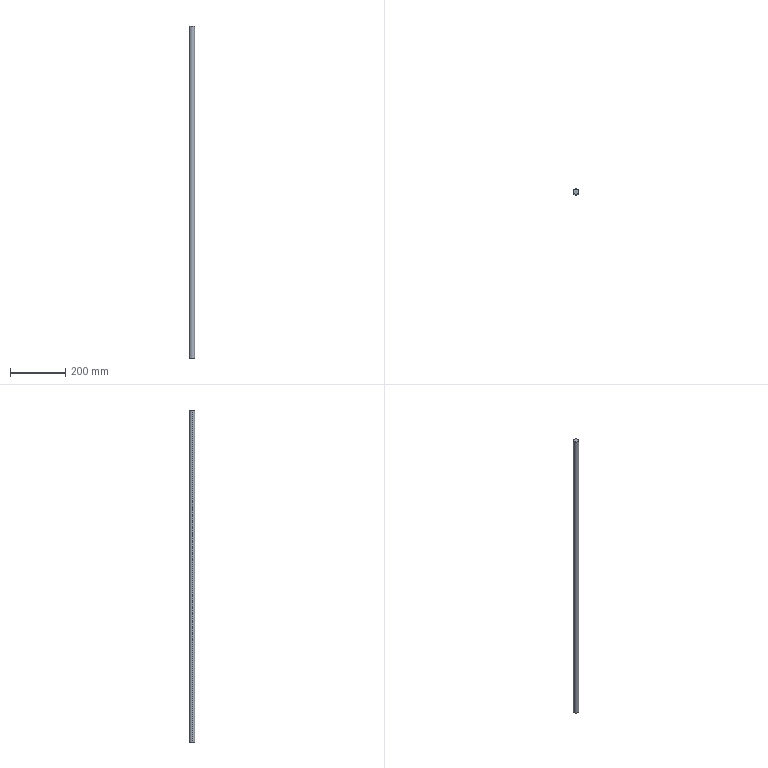Part | SolidWorks | features Extrusion 1, ICE 1 | 1 solid | 28 faces | box 20 x 20 x 1198 mm | volume 373288 mm3 | cylinder 14 | plane 14 | commonest cylinder face diameters 6 x12 20 x2
STEP:
#1=CARTESIAN_POINT('',(0.,6.5,-504.));
#2=VERTEX_POINT('',#1);
#3=CARTESIAN_POINT('',(3.,6.5,-507.));
#4=VERTEX_POINT('',#3);
#5=CARTESIAN_POINT('',(0.,6.5,-507.));
#6=DIRECTION('',(0.,1.,0.));
#7=DIRECTION('',(0.,0.,1.));
#8=AXIS2_PLACEMENT_3D('',#5,#6,#7);
#9=CIRCLE('',#8,3.);
#10=EDGE_CURVE('',#2,#4,#9,.T.);
#11=ORIENTED_EDGE('',*,*,#10,.F.);
#12=CARTESIAN_POINT('',(0.,10.,-504.));
#13=VERTEX_POINT('',#12);
#14=CARTESIAN_POINT('',(0.,6.5,-504.));
#15=DIRECTION('',(0.,1.,0.));
#16=VECTOR('',#15,1000.);
#17=LINE('',#14,#16);
#18=EDGE_CURVE('',#2,#13,#17,.T.);
#19=ORIENTED_EDGE('',*,*,#18,.T.);
#20=CARTESIAN_POINT('',(3.,9.539,-507.));
#21=VERTEX_POINT('',#20);
#22=CARTESIAN_POINT('',(3.,9.539,-507.));
#23=CARTESIAN_POINT('',(3.,9.539,-506.802));
#24=CARTESIAN_POINT('',(2.981,9.546,-506.607));
#25=CARTESIAN_POINT('',(2.904,9.569,-506.22));
#26=CARTESIAN_POINT('',(2.845,9.587,-506.029));
#27=CARTESIAN_POINT('',(2.62,9.652,-505.487));
#28=CARTESIAN_POINT('',(2.397,9.713,-505.155));
#29=CARTESIAN_POINT('',(1.985,9.802,-504.742));
#30=CARTESIAN_POINT('',(1.832,9.832,-504.616));
#31=CARTESIAN_POINT('',(1.506,9.887,-504.398));
#32=CARTESIAN_POINT('',(1.335,9.912,-504.306));
#33=CARTESIAN_POINT('',(0.973,9.954,-504.155));
#34=CARTESIAN_POINT('',(0.7814,9.971,-504.097));
#35=CARTESIAN_POINT('',(0.3955,9.994,-504.02));
#36=CARTESIAN_POINT('',(0.1994,10.,-504.));
#37=CARTESIAN_POINT('',(0.,10.,-504.));
#38=B_SPLINE_CURVE_WITH_KNOTS('',3,(#22,#23,#24,#25,#26,#27,#28,#29,#30,#31,#32,#33,#34,#35,#36,#37),.UNSPECIFIED.,.F.,.F.,(4,2,2,2,2,2,2,4),(0.01415,0.01474,0.01533,0.01651,0.0171,0.01769,0.01828,0.01887),.UNSPECIFIED.);
#39=EDGE_CURVE('',#21,#13,#38,.T.);
#40=ORIENTED_EDGE('',*,*,#39,.F.);
#41=CARTESIAN_POINT('',(3.,6.5,-507.));
#42=DIRECTION('',(0.,1.,0.));
#43=VECTOR('',#42,1000.);
#44=LINE('',#41,#43);
#45=EDGE_CURVE('',#4,#21,#44,.T.);
#46=ORIENTED_EDGE('',*,*,#45,.F.);
#47=EDGE_LOOP('',(#11,#19,#40,#46));
#48=FACE_OUTER_BOUND('',#47,.T.);
#49=CARTESIAN_POINT('',(0.,6.5,-507.));
#50=DIRECTION('',(0.,1.,0.));
#51=DIRECTION('',(0.,0.,1.));
#52=AXIS2_PLACEMENT_3D('',#49,#50,#51);
#53=CYLINDRICAL_SURFACE('',#52,3.);
#54=ADVANCED_FACE('',(#48),#53,.F.);
#55=CARTESIAN_POINT('',(0.,6.5,24.));
#56=VERTEX_POINT('',#55);
#57=CARTESIAN_POINT('',(3.,6.5,21.));
#58=VERTEX_POINT('',#57);
#59=CARTESIAN_POINT('',(0.,6.5,21.));
#60=DIRECTION('',(0.,1.,0.));
#61=DIRECTION('',(0.,0.,1.));
#62=AXIS2_PLACEMENT_3D('',#59,#60,#61);
#63=CIRCLE('',#62,3.);
#64=EDGE_CURVE('',#56,#58,#63,.T.);
#65=ORIENTED_EDGE('',*,*,#64,.F.);
#66=CARTESIAN_POINT('',(0.,10.,24.));
#67=VERTEX_POINT('',#66);
#68=CARTESIAN_POINT('',(0.,6.5,24.));
#69=DIRECTION('',(0.,1.,0.));
#70=VECTOR('',#69,1000.);
#71=LINE('',#68,#70);
#72=EDGE_CURVE('',#56,#67,#71,.T.);
#73=ORIENTED_EDGE('',*,*,#72,.T.);
#74=CARTESIAN_POINT('',(3.,9.539,21.));
#75=VERTEX_POINT('',#74);
#76=CARTESIAN_POINT('',(3.,9.539,21.));
#77=CARTESIAN_POINT('',(3.,9.539,21.198));
#78=CARTESIAN_POINT('',(2.981,9.546,21.393));
#79=CARTESIAN_POINT('',(2.904,9.569,21.78));
#80=CARTESIAN_POINT('',(2.845,9.587,21.971));
#81=CARTESIAN_POINT('',(2.62,9.652,22.513));
#82=CARTESIAN_POINT('',(2.397,9.713,22.845));
#83=CARTESIAN_POINT('',(1.985,9.802,23.258));
#84=CARTESIAN_POINT('',(1.832,9.832,23.384));
#85=CARTESIAN_POINT('',(1.506,9.887,23.602));
#86=CARTESIAN_POINT('',(1.335,9.912,23.694));
#87=CARTESIAN_POINT('',(0.973,9.954,23.845));
#88=CARTESIAN_POINT('',(0.7814,9.971,23.903));
#89=CARTESIAN_POINT('',(0.3955,9.994,23.98));
#90=CARTESIAN_POINT('',(0.1994,10.,24.));
#91=CARTESIAN_POINT('',(0.,10.,24.));
#92=B_SPLINE_CURVE_WITH_KNOTS('',3,(#76,#77,#78,#79,#80,#81,#82,#83,#84,#85,#86,#87,#88,#89,#90,#91),.UNSPECIFIED.,.F.,.F.,(4,2,2,2,2,2,2,4),(0.01415,0.01474,0.01533,0.01651,0.0171,0.01769,0.01828,0.01887),.UNSPECIFIED.);
#93=EDGE_CURVE('',#75,#67,#92,.T.);
#94=ORIENTED_EDGE('',*,*,#93,.F.);
#95=CARTESIAN_POINT('',(3.,6.5,21.));
#96=DIRECTION('',(0.,1.,0.));
#97=VECTOR('',#96,1000.);
#98=LINE('',#95,#97);
#99=EDGE_CURVE('',#58,#75,#98,.T.);
#100=ORIENTED_EDGE('',*,*,#99,.F.);
#101=EDGE_LOOP('',(#65,#73,#94,#100));
#102=FACE_OUTER_BOUND('',#101,.T.);
#103=CARTESIAN_POINT('',(0.,6.5,21.));
#104=DIRECTION('',(0.,1.,0.));
#105=DIRECTION('',(0.,0.,1.));
#106=AXIS2_PLACEMENT_3D('',#103,#104,#105);
#107=CYLINDRICAL_SURFACE('',#106,3.);
#108=ADVANCED_FACE('',(#102),#107,.F.);
#109=CARTESIAN_POINT('',(0.,6.5,-417.));
#110=VERTEX_POINT('',#109);
#111=CARTESIAN_POINT('',(3.,6.5,-420.));
#112=VERTEX_POINT('',#111);
#113=CARTESIAN_POINT('',(0.,6.5,-420.));
#114=DIRECTION('',(0.,1.,0.));
#115=DIRECTION('',(0.,0.,1.));
#116=AXIS2_PLACEMENT_3D('',#113,#114,#115);
#117=CIRCLE('',#116,3.);
#118=EDGE_CURVE('',#110,#112,#117,.T.);
#119=ORIENTED_EDGE('',*,*,#118,.F.);
#120=CARTESIAN_POINT('',(0.,10.,-417.));
#121=VERTEX_POINT('',#120);
#122=CARTESIAN_POINT('',(0.,6.5,-417.));
#123=DIRECTION('',(0.,1.,0.));
#124=VECTOR('',#123,1000.);
#125=LINE('',#122,#124);
#126=EDGE_CURVE('',#110,#121,#125,.T.);
#127=ORIENTED_EDGE('',*,*,#126,.T.);
#128=CARTESIAN_POINT('',(3.,9.539,-420.));
#129=VERTEX_POINT('',#128);
#130=CARTESIAN_POINT('',(3.,9.539,-420.));
#131=CARTESIAN_POINT('',(3.,9.539,-419.802));
#132=CARTESIAN_POINT('',(2.981,9.546,-419.607));
#133=CARTESIAN_POINT('',(2.904,9.569,-419.22));
#134=CARTESIAN_POINT('',(2.845,9.587,-419.029));
#135=CARTESIAN_POINT('',(2.62,9.652,-418.487));
#136=CARTESIAN_POINT('',(2.397,9.713,-418.155));
#137=CARTESIAN_POINT('',(1.985,9.802,-417.742));
#138=CARTESIAN_POINT('',(1.832,9.832,-417.616));
#139=CARTESIAN_POINT('',(1.506,9.887,-417.398));
#140=CARTESIAN_POINT('',(1.335,9.912,-417.306));
#141=CARTESIAN_POINT('',(0.973,9.954,-417.155));
#142=CARTESIAN_POINT('',(0.7814,9.971,-417.097));
#143=CARTESIAN_POINT('',(0.3955,9.994,-417.02));
#144=CARTESIAN_POINT('',(0.1994,10.,-417.));
#145=CARTESIAN_POINT('',(0.,10.,-417.));
#146=B_SPLINE_CURVE_WITH_KNOTS('',3,(#130,#131,#132,#133,#134,#135,#136,#137,#138,#139,#140,#141,#142,#143,#144,#145),.UNSPECIFIED.,.F.,.F.,(4,2,2,2,2,2,2,4),(0.01415,0.01474,0.01533,0.01651,0.0171,0.01769,0.01828,0.01887),.UNSPECIFIED.);
#147=EDGE_CURVE('',#129,#121,#146,.T.);
#148=ORIENTED_EDGE('',*,*,#147,.F.);
#149=CARTESIAN_POINT('',(3.,6.5,-420.));
#150=DIRECTION('',(0.,1.,0.));
#151=VECTOR('',#150,1000.);
#152=LINE('',#149,#151);
#153=EDGE_CURVE('',#112,#129,#152,.T.);
#154=ORIENTED_EDGE('',*,*,#153,.F.);
#155=EDGE_LOOP('',(#119,#127,#148,#154));
#156=FACE_OUTER_BOUND('',#155,.T.);
#157=CARTESIAN_POINT('',(0.,6.5,-420.));
#158=DIRECTION('',(0.,1.,0.));
#159=DIRECTION('',(0.,0.,1.));
#160=AXIS2_PLACEMENT_3D('',#157,#158,#159);
#161=CYLINDRICAL_SURFACE('',#160,3.);
#162=ADVANCED_FACE('',(#156),#161,.F.);
#163=CARTESIAN_POINT('',(0.,6.5,548.));
#164=VERTEX_POINT('',#163);
#165=CARTESIAN_POINT('',(3.,6.5,545.));
#166=VERTEX_POINT('',#165);
#167=CARTESIAN_POINT('',(0.,6.5,545.));
#168=DIRECTION('',(0.,1.,0.));
#169=DIRECTION('',(0.,0.,-1.));
#170=AXIS2_PLACEMENT_3D('',#167,#168,#169);
#171=CIRCLE('',#170,3.);
#172=EDGE_CURVE('',#164,#166,#171,.T.);
#173=ORIENTED_EDGE('',*,*,#172,.F.);
#174=CARTESIAN_POINT('',(0.,10.,548.));
#175=VERTEX_POINT('',#174);
#176=CARTESIAN_POINT('',(0.,6.5,548.));
#177=DIRECTION('',(0.,1.,0.));
#178=VECTOR('',#177,1000.);
#179=LINE('',#176,#178);
#180=EDGE_CURVE('',#164,#175,#179,.T.);
#181=ORIENTED_EDGE('',*,*,#180,.T.);
#182=CARTESIAN_POINT('',(3.,9.539,545.));
#183=VERTEX_POINT('',#182);
#184=CARTESIAN_POINT('',(3.,9.539,545.));
#185=CARTESIAN_POINT('',(3.,9.539,545.198));
#186=CARTESIAN_POINT('',(2.981,9.546,545.393));
#187=CARTESIAN_POINT('',(2.904,9.569,545.78));
#188=CARTESIAN_POINT('',(2.845,9.587,545.971));
#189=CARTESIAN_POINT('',(2.62,9.652,546.513));
#190=CARTESIAN_POINT('',(2.397,9.713,546.845));
#191=CARTESIAN_POINT('',(1.985,9.802,547.258));
#192=CARTESIAN_POINT('',(1.832,9.832,547.384));
#193=CARTESIAN_POINT('',(1.506,9.887,547.602));
#194=CARTESIAN_POINT('',(1.335,9.912,547.694));
#195=CARTESIAN_POINT('',(0.973,9.954,547.845));
#196=CARTESIAN_POINT('',(0.7814,9.971,547.903));
#197=CARTESIAN_POINT('',(0.3955,9.994,547.98));
#198=CARTESIAN_POINT('',(0.1994,10.,548.));
#199=CARTESIAN_POINT('',(0.,10.,548.));
#200=B_SPLINE_CURVE_WITH_KNOTS('',3,(#184,#185,#186,#187,#188,#189,#190,#191,#192,#193,#194,#195,#196,#197,#198,#199),.UNSPECIFIED.,.F.,.F.,(4,2,2,2,2,2,2,4),(0.01415,0.01474,0.01533,0.01651,0.0171,0.01769,0.01828,0.01887),.UNSPECIFIED.);
#201=EDGE_CURVE('',#183,#175,#200,.T.);
#202=ORIENTED_EDGE('',*,*,#201,.F.);
#203=CARTESIAN_POINT('',(3.,6.5,545.));
#204=DIRECTION('',(0.,1.,0.));
#205=VECTOR('',#204,1000.);
#206=LINE('',#203,#205);
#207=EDGE_CURVE('',#166,#183,#206,.T.);
#208=ORIENTED_EDGE('',*,*,#207,.F.);
#209=EDGE_LOOP('',(#173,#181,#202,#208));
#210=FACE_OUTER_BOUND('',#209,.T.);
#211=CARTESIAN_POINT('',(0.,6.5,545.));
#212=DIRECTION('',(0.,1.,0.));
#213=DIRECTION('',(0.,0.,1.));
#214=AXIS2_PLACEMENT_3D('',#211,#212,#213);
#215=CYLINDRICAL_SURFACE('',#214,3.);
#216=ADVANCED_FACE('',(#210),#215,.F.);
#217=ORIENTED_EDGE('',*,*,#39,.T.);
#218=CARTESIAN_POINT('',(-3.,9.539,-507.));
#219=VERTEX_POINT('',#218);
#220=CARTESIAN_POINT('',(0.,10.,-504.));
#221=CARTESIAN_POINT('',(-0.1995,10.,-504.));
#222=CARTESIAN_POINT('',(-0.3955,9.994,-504.02));
#223=CARTESIAN_POINT('',(-0.7806,9.971,-504.097));
#224=CARTESIAN_POINT('',(-0.9719,9.954,-504.155));
#225=CARTESIAN_POINT('',(-1.335,9.912,-504.306));
#226=CARTESIAN_POINT('',(-1.507,9.887,-504.398));
#227=CARTESIAN_POINT('',(-1.832,9.832,-504.616));
#228=CARTESIAN_POINT('',(-1.985,9.802,-504.742));
#229=CARTESIAN_POINT('',(-2.398,9.712,-505.155));
#230=CARTESIAN_POINT('',(-2.62,9.652,-505.488));
#231=CARTESIAN_POINT('',(-2.845,9.587,-506.029));
#232=CARTESIAN_POINT('',(-2.903,9.569,-506.22));
#233=CARTESIAN_POINT('',(-2.981,9.546,-506.607));
#234=CARTESIAN_POINT('',(-3.,9.539,-506.803));
#235=CARTESIAN_POINT('',(-3.,9.539,-507.));
#236=B_SPLINE_CURVE_WITH_KNOTS('',3,(#220,#221,#222,#223,#224,#225,#226,#227,#228,#229,#230,#231,#232,#233,#234,#235),.UNSPECIFIED.,.F.,.F.,(4,2,2,2,2,2,2,4),(0.,0.0005898,0.00118,0.001769,0.002359,0.003539,0.004129,0.004718),.UNSPECIFIED.);
#237=EDGE_CURVE('',#13,#219,#236,.T.);
#238=ORIENTED_EDGE('',*,*,#237,.T.);
#239=CARTESIAN_POINT('',(-3.,9.539,-545.));
#240=VERTEX_POINT('',#239);
#241=CARTESIAN_POINT('',(-3.,9.539,599.));
#242=DIRECTION('',(0.,0.,-1.));
#243=VECTOR('',#242,1000.);
#244=LINE('',#241,#243);
#245=EDGE_CURVE('',#219,#240,#244,.T.);
#246=ORIENTED_EDGE('',*,*,#245,.T.);
#247=CARTESIAN_POINT('',(3.,9.539,-545.));
#248=VERTEX_POINT('',#247);
#249=CARTESIAN_POINT('',(-3.,9.539,-545.));
#250=CARTESIAN_POINT('',(-3.,9.539,-545.197));
#251=CARTESIAN_POINT('',(-2.98,9.546,-545.397));
#252=CARTESIAN_POINT('',(-2.903,9.57,-545.783));
#253=CARTESIAN_POINT('',(-2.846,9.587,-545.97));
#254=CARTESIAN_POINT('',(-2.694,9.631,-546.335));
#255=CARTESIAN_POINT('',(-2.601,9.657,-546.508));
#256=CARTESIAN_POINT('',(-2.384,9.712,-546.832));
#257=CARTESIAN_POINT('',(-2.259,9.743,-546.984));
#258=CARTESIAN_POINT('',(-1.982,9.803,-547.261));
#259=CARTESIAN_POINT('',(-1.831,9.832,-547.384));
#260=CARTESIAN_POINT('',(-1.507,9.887,-547.601));
#261=CARTESIAN_POINT('',(-1.331,9.913,-547.695));
#262=CARTESIAN_POINT('',(-0.9699,9.955,-547.846));
#263=CARTESIAN_POINT('',(-0.7828,9.971,-547.903));
#264=CARTESIAN_POINT('',(-0.3953,9.994,-547.98));
#265=CARTESIAN_POINT('',(-0.1963,10.,-548.));
#266=CARTESIAN_POINT('',(0.1967,10.,-548.));
#267=CARTESIAN_POINT('',(0.3937,9.994,-547.981));
#268=CARTESIAN_POINT('',(0.7832,9.971,-547.903));
#269=CARTESIAN_POINT('',(0.9708,9.954,-547.845));
#270=CARTESIAN_POINT('',(1.332,9.913,-547.695));
#271=CARTESIAN_POINT('',(1.508,9.887,-547.601));
#272=CARTESIAN_POINT('',(1.833,9.832,-547.383));
#273=CARTESIAN_POINT('',(1.983,9.802,-547.26));
#274=CARTESIAN_POINT('',(2.26,9.742,-546.983));
#275=CARTESIAN_POINT('',(2.385,9.712,-546.83));
#276=CARTESIAN_POINT('',(2.601,9.656,-546.507));
#277=CARTESIAN_POINT('',(2.694,9.631,-546.335));
#278=CARTESIAN_POINT('',(2.846,9.587,-545.969));
#279=CARTESIAN_POINT('',(2.903,9.569,-545.782));
#280=CARTESIAN_POINT('',(2.98,9.546,-545.397));
#281=CARTESIAN_POINT('',(3.,9.539,-545.198));
#282=CARTESIAN_POINT('',(3.,9.539,-545.));
#283=B_SPLINE_CURVE_WITH_KNOTS('',3,(#249,#250,#251,#252,#253,#254,#255,#256,#257,#258,#259,#260,#261,#262,#263,#264,#265,#266,#267,#268,#269,#270,#271,#272,#273,#274,#275,#276,#277,#278,#279,#280,#281,#282),.UNSPECIFIED.,.F.,.F.,(4,2,2,2,2,2,2,2,2,2,2,2,2,2,2,2,4),(0.004718,0.005308,0.005897,0.006487,0.007076,0.007666,0.008255,0.008845,0.009434,0.01002,0.01061,0.0112,0.01179,0.01238,0.01297,0.01356,0.01415),.UNSPECIFIED.);
#284=EDGE_CURVE('',#240,#248,#283,.T.);
#285=ORIENTED_EDGE('',*,*,#284,.T.);
#286=CARTESIAN_POINT('',(3.,9.539,599.));
#287=DIRECTION('',(0.,0.,1.));
#288=VECTOR('',#287,1000.);
#289=LINE('',#286,#288);
#290=EDGE_CURVE('',#248,#21,#289,.T.);
#291=ORIENTED_EDGE('',*,*,#290,.T.);
#292=EDGE_LOOP('',(#217,#238,#246,#285,#291));
#293=FACE_BOUND('',#292,.T.);
#294=ORIENTED_EDGE('',*,*,#93,.T.);
#295=CARTESIAN_POINT('',(-3.,9.539,21.));
#296=VERTEX_POINT('',#295);
#297=CARTESIAN_POINT('',(0.,10.,24.));
#298=CARTESIAN_POINT('',(-0.1995,10.,24.));
#299=CARTESIAN_POINT('',(-0.3955,9.994,23.98));
#300=CARTESIAN_POINT('',(-0.7806,9.971,23.903));
#301=CARTESIAN_POINT('',(-0.9719,9.954,23.845));
#302=CARTESIAN_POINT('',(-1.335,9.912,23.694));
#303=CARTESIAN_POINT('',(-1.507,9.887,23.602));
#304=CARTESIAN_POINT('',(-1.832,9.832,23.384));
#305=CARTESIAN_POINT('',(-1.985,9.802,23.258));
#306=CARTESIAN_POINT('',(-2.398,9.712,22.845));
#307=CARTESIAN_POINT('',(-2.62,9.652,22.512));
#308=CARTESIAN_POINT('',(-2.845,9.587,21.971));
#309=CARTESIAN_POINT('',(-2.903,9.569,21.78));
#310=CARTESIAN_POINT('',(-2.981,9.546,21.393));
#311=CARTESIAN_POINT('',(-3.,9.539,21.197));
#312=CARTESIAN_POINT('',(-3.,9.539,21.));
#313=B_SPLINE_CURVE_WITH_KNOTS('',3,(#297,#298,#299,#300,#301,#302,#303,#304,#305,#306,#307,#308,#309,#310,#311,#312),.UNSPECIFIED.,.F.,.F.,(4,2,2,2,2,2,2,4),(0.,0.0005898,0.00118,0.001769,0.002359,0.003539,0.004129,0.004718),.UNSPECIFIED.);
#314=EDGE_CURVE('',#67,#296,#313,.T.);
#315=ORIENTED_EDGE('',*,*,#314,.T.);
#316=CARTESIAN_POINT('',(-3.,9.539,-17.));
#317=VERTEX_POINT('',#316);
#318=CARTESIAN_POINT('',(-3.,9.539,599.));
#319=DIRECTION('',(0.,0.,-1.));
#320=VECTOR('',#319,1000.);
#321=LINE('',#318,#320);
#322=EDGE_CURVE('',#296,#317,#321,.T.);
#323=ORIENTED_EDGE('',*,*,#322,.T.);
#324=CARTESIAN_POINT('',(3.,9.539,-17.));
#325=VERTEX_POINT('',#324);
#326=CARTESIAN_POINT('',(-3.,9.539,-17.));
#327=CARTESIAN_POINT('',(-3.,9.539,-17.197));
#328=CARTESIAN_POINT('',(-2.98,9.546,-17.397));
#329=CARTESIAN_POINT('',(-2.903,9.57,-17.783));
#330=CARTESIAN_POINT('',(-2.846,9.587,-17.97));
#331=CARTESIAN_POINT('',(-2.694,9.631,-18.335));
#332=CARTESIAN_POINT('',(-2.601,9.657,-18.508));
#333=CARTESIAN_POINT('',(-2.384,9.712,-18.832));
#334=CARTESIAN_POINT('',(-2.259,9.743,-18.984));
#335=CARTESIAN_POINT('',(-1.982,9.803,-19.261));
#336=CARTESIAN_POINT('',(-1.831,9.832,-19.384));
#337=CARTESIAN_POINT('',(-1.507,9.887,-19.601));
#338=CARTESIAN_POINT('',(-1.331,9.913,-19.695));
#339=CARTESIAN_POINT('',(-0.9699,9.955,-19.846));
#340=CARTESIAN_POINT('',(-0.7828,9.971,-19.903));
#341=CARTESIAN_POINT('',(-0.3953,9.994,-19.98));
#342=CARTESIAN_POINT('',(-0.1963,10.,-20.));
#343=CARTESIAN_POINT('',(0.1967,10.,-20.));
#344=CARTESIAN_POINT('',(0.3937,9.994,-19.981));
#345=CARTESIAN_POINT('',(0.7832,9.971,-19.903));
#346=CARTESIAN_POINT('',(0.9708,9.954,-19.845));
#347=CARTESIAN_POINT('',(1.332,9.913,-19.695));
#348=CARTESIAN_POINT('',(1.508,9.887,-19.601));
#349=CARTESIAN_POINT('',(1.833,9.832,-19.383));
#350=CARTESIAN_POINT('',(1.983,9.802,-19.26));
#351=CARTESIAN_POINT('',(2.26,9.742,-18.983));
#352=CARTESIAN_POINT('',(2.385,9.712,-18.83));
#353=CARTESIAN_POINT('',(2.601,9.656,-18.507));
#354=CARTESIAN_POINT('',(2.694,9.631,-18.335));
#355=CARTESIAN_POINT('',(2.846,9.587,-17.969));
#356=CARTESIAN_POINT('',(2.903,9.569,-17.782));
#357=CARTESIAN_POINT('',(2.98,9.546,-17.397));
#358=CARTESIAN_POINT('',(3.,9.539,-17.198));
#359=CARTESIAN_POINT('',(3.,9.539,-17.));
#360=B_SPLINE_CURVE_WITH_KNOTS('',3,(#326,#327,#328,#329,#330,#331,#332,#333,#334,#335,#336,#337,#338,#339,#340,#341,#342,#343,#344,#345,#346,#347,#348,#349,#350,#351,#352,#353,#354,#355,#356,#357,#358,#359),.UNSPECIFIED.,.F.,.F.,(4,2,2,2,2,2,2,2,2,2,2,2,2,2,2,2,4),(0.004718,0.005308,0.005897,0.006487,0.007076,0.007666,0.008255,0.008845,0.009434,0.01002,0.01061,0.0112,0.01179,0.01238,0.01297,0.01356,0.01415),.UNSPECIFIED.);
#361=EDGE_CURVE('',#317,#325,#360,.T.);
#362=ORIENTED_EDGE('',*,*,#361,.T.);
#363=CARTESIAN_POINT('',(3.,9.539,599.));
#364=DIRECTION('',(0.,0.,1.));
#365=VECTOR('',#364,1000.);
#366=LINE('',#363,#365);
#367=EDGE_CURVE('',#325,#75,#366,.T.);
#368=ORIENTED_EDGE('',*,*,#367,.T.);
#369=EDGE_LOOP('',(#294,#315,#323,#362,#368));
#370=FACE_BOUND('',#369,.T.);
#371=ORIENTED_EDGE('',*,*,#147,.T.);
#372=CARTESIAN_POINT('',(-3.,9.539,-420.));
#373=VERTEX_POINT('',#372);
#374=CARTESIAN_POINT('',(0.,10.,-417.));
#375=CARTESIAN_POINT('',(-0.1995,10.,-417.));
#376=CARTESIAN_POINT('',(-0.3955,9.994,-417.02));
#377=CARTESIAN_POINT('',(-0.7806,9.971,-417.097));
#378=CARTESIAN_POINT('',(-0.9719,9.954,-417.155));
#379=CARTESIAN_POINT('',(-1.335,9.912,-417.306));
#380=CARTESIAN_POINT('',(-1.507,9.887,-417.398));
#381=CARTESIAN_POINT('',(-1.832,9.832,-417.616));
#382=CARTESIAN_POINT('',(-1.985,9.802,-417.742));
#383=CARTESIAN_POINT('',(-2.398,9.712,-418.155));
#384=CARTESIAN_POINT('',(-2.62,9.652,-418.488));
#385=CARTESIAN_POINT('',(-2.845,9.587,-419.029));
#386=CARTESIAN_POINT('',(-2.903,9.569,-419.22));
#387=CARTESIAN_POINT('',(-2.981,9.546,-419.607));
#388=CARTESIAN_POINT('',(-3.,9.539,-419.803));
#389=CARTESIAN_POINT('',(-3.,9.539,-420.));
#390=B_SPLINE_CURVE_WITH_KNOTS('',3,(#374,#375,#376,#377,#378,#379,#380,#381,#382,#383,#384,#385,#386,#387,#388,#389),.UNSPECIFIED.,.F.,.F.,(4,2,2,2,2,2,2,4),(0.,0.0005898,0.00118,0.001769,0.002359,0.003539,0.004129,0.004718),.UNSPECIFIED.);
#391=EDGE_CURVE('',#121,#373,#390,.T.);
#392=ORIENTED_EDGE('',*,*,#391,.T.);
#393=CARTESIAN_POINT('',(-3.,9.539,-440.));
#394=VERTEX_POINT('',#393);
#395=CARTESIAN_POINT('',(-3.,9.539,599.));
#396=DIRECTION('',(0.,0.,-1.));
#397=VECTOR('',#396,1000.);
#398=LINE('',#395,#397);
#399=EDGE_CURVE('',#373,#394,#398,.T.);
#400=ORIENTED_EDGE('',*,*,#399,.T.);
#401=CARTESIAN_POINT('',(3.,9.539,-440.));
#402=VERTEX_POINT('',#401);
#403=CARTESIAN_POINT('',(-3.,9.539,-440.));
#404=CARTESIAN_POINT('',(-3.,9.539,-440.199));
#405=CARTESIAN_POINT('',(-2.98,9.546,-440.395));
#406=CARTESIAN_POINT('',(-2.903,9.569,-440.78));
#407=CARTESIAN_POINT('',(-2.845,9.587,-440.971));
#408=CARTESIAN_POINT('',(-2.694,9.631,-441.334));
#409=CARTESIAN_POINT('',(-2.602,9.656,-441.506));
#410=CARTESIAN_POINT('',(-2.385,9.712,-441.831));
#411=CARTESIAN_POINT('',(-2.259,9.743,-441.984));
#412=CARTESIAN_POINT('',(-1.847,9.832,-442.396));
#413=CARTESIAN_POINT('',(-1.514,9.891,-442.619));
#414=CARTESIAN_POINT('',(-0.9732,9.954,-442.844));
#415=CARTESIAN_POINT('',(-0.783,9.971,-442.903));
#416=CARTESIAN_POINT('',(-0.3953,9.994,-442.98));
#417=CARTESIAN_POINT('',(-0.1999,10.,-443.));
#418=CARTESIAN_POINT('',(0.194,10.,-443.));
#419=CARTESIAN_POINT('',(0.394,9.994,-442.981));
#420=CARTESIAN_POINT('',(0.7797,9.971,-442.904));
#421=CARTESIAN_POINT('',(0.9673,9.955,-442.847));
#422=CARTESIAN_POINT('',(1.332,9.913,-442.695));
#423=CARTESIAN_POINT('',(1.506,9.887,-442.602));
#424=CARTESIAN_POINT('',(1.83,9.833,-442.386));
#425=CARTESIAN_POINT('',(1.982,9.803,-442.26));
#426=CARTESIAN_POINT('',(2.259,9.743,-441.984));
#427=CARTESIAN_POINT('',(2.383,9.713,-441.833));
#428=CARTESIAN_POINT('',(2.6,9.657,-441.51));
#429=CARTESIAN_POINT('',(2.694,9.631,-441.334));
#430=CARTESIAN_POINT('',(2.845,9.587,-440.973));
#431=CARTESIAN_POINT('',(2.902,9.57,-440.786));
#432=CARTESIAN_POINT('',(2.98,9.546,-440.399));
#433=CARTESIAN_POINT('',(3.,9.539,-440.199));
#434=CARTESIAN_POINT('',(3.,9.539,-440.));
#435=B_SPLINE_CURVE_WITH_KNOTS('',3,(#403,#404,#405,#406,#407,#408,#409,#410,#411,#412,#413,#414,#415,#416,#417,#418,#419,#420,#421,#422,#423,#424,#425,#426,#427,#428,#429,#430,#431,#432,#433,#434),.UNSPECIFIED.,.F.,.F.,(4,2,2,2,2,2,2,2,2,2,2,2,2,2,2,4),(0.,0.0005894,0.001179,0.001768,0.002358,0.003536,0.004126,0.004715,0.005305,0.005894,0.006484,0.007073,0.007662,0.008252,0.008841,0.009431),.UNSPECIFIED.);
#436=EDGE_CURVE('',#394,#402,#435,.T.);
#437=ORIENTED_EDGE('',*,*,#436,.T.);
#438=CARTESIAN_POINT('',(3.,9.539,599.));
#439=DIRECTION('',(0.,0.,1.));
#440=VECTOR('',#439,1000.);
#441=LINE('',#438,#440);
#442=EDGE_CURVE('',#402,#129,#441,.T.);
#443=ORIENTED_EDGE('',*,*,#442,.T.);
#444=EDGE_LOOP('',(#371,#392,#400,#437,#443));
#445=FACE_BOUND('',#444,.T.);
#446=ORIENTED_EDGE('',*,*,#201,.T.);
#447=CARTESIAN_POINT('',(-3.,9.539,545.));
#448=VERTEX_POINT('',#447);
#449=CARTESIAN_POINT('',(0.,10.,548.));
#450=CARTESIAN_POINT('',(-0.1995,10.,548.));
#451=CARTESIAN_POINT('',(-0.3955,9.994,547.98));
#452=CARTESIAN_POINT('',(-0.7806,9.971,547.903));
#453=CARTESIAN_POINT('',(-0.9719,9.954,547.845));
#454=CARTESIAN_POINT('',(-1.335,9.912,547.694));
#455=CARTESIAN_POINT('',(-1.507,9.887,547.602));
#456=CARTESIAN_POINT('',(-1.832,9.832,547.384));
#457=CARTESIAN_POINT('',(-1.985,9.802,547.258));
#458=CARTESIAN_POINT('',(-2.398,9.712,546.845));
#459=CARTESIAN_POINT('',(-2.62,9.652,546.512));
#460=CARTESIAN_POINT('',(-2.845,9.587,545.971));
#461=CARTESIAN_POINT('',(-2.903,9.569,545.78));
#462=CARTESIAN_POINT('',(-2.981,9.546,545.393));
#463=CARTESIAN_POINT('',(-3.,9.539,545.197));
#464=CARTESIAN_POINT('',(-3.,9.539,545.));
#465=B_SPLINE_CURVE_WITH_KNOTS('',3,(#449,#450,#451,#452,#453,#454,#455,#456,#457,#458,#459,#460,#461,#462,#463,#464),.UNSPECIFIED.,.F.,.F.,(4,2,2,2,2,2,2,4),(0.,0.0005898,0.00118,0.001769,0.002359,0.003539,0.004129,0.004718),.UNSPECIFIED.);
#466=EDGE_CURVE('',#175,#448,#465,.T.);
#467=ORIENTED_EDGE('',*,*,#466,.T.);
#468=CARTESIAN_POINT('',(-3.,9.539,507.));
#469=VERTEX_POINT('',#468);
#470=CARTESIAN_POINT('',(-3.,9.539,599.));
#471=DIRECTION('',(0.,0.,-1.));
#472=VECTOR('',#471,1000.);
#473=LINE('',#470,#472);
#474=EDGE_CURVE('',#448,#469,#473,.T.);
#475=ORIENTED_EDGE('',*,*,#474,.T.);
#476=CARTESIAN_POINT('',(3.,9.539,507.));
#477=VERTEX_POINT('',#476);
#478=CARTESIAN_POINT('',(-3.,9.539,507.));
#479=CARTESIAN_POINT('',(-3.,9.539,506.801));
#480=CARTESIAN_POINT('',(-2.98,9.546,506.605));
#481=CARTESIAN_POINT('',(-2.903,9.569,506.22));
#482=CARTESIAN_POINT('',(-2.845,9.587,506.029));
#483=CARTESIAN_POINT('',(-2.694,9.631,505.666));
#484=CARTESIAN_POINT('',(-2.602,9.656,505.494));
#485=CARTESIAN_POINT('',(-2.385,9.712,505.169));
#486=CARTESIAN_POINT('',(-2.259,9.743,505.016));
#487=CARTESIAN_POINT('',(-1.847,9.832,504.604));
#488=CARTESIAN_POINT('',(-1.514,9.891,504.381));
#489=CARTESIAN_POINT('',(-0.9732,9.954,504.156));
#490=CARTESIAN_POINT('',(-0.783,9.971,504.097));
#491=CARTESIAN_POINT('',(-0.3953,9.994,504.02));
#492=CARTESIAN_POINT('',(-0.1999,10.,504.));
#493=CARTESIAN_POINT('',(0.194,10.,504.));
#494=CARTESIAN_POINT('',(0.394,9.994,504.019));
#495=CARTESIAN_POINT('',(0.7797,9.971,504.096));
#496=CARTESIAN_POINT('',(0.9673,9.955,504.153));
#497=CARTESIAN_POINT('',(1.332,9.913,504.305));
#498=CARTESIAN_POINT('',(1.506,9.887,504.398));
#499=CARTESIAN_POINT('',(1.83,9.833,504.614));
#500=CARTESIAN_POINT('',(1.982,9.803,504.74));
#501=CARTESIAN_POINT('',(2.259,9.743,505.016));
#502=CARTESIAN_POINT('',(2.383,9.713,505.167));
#503=CARTESIAN_POINT('',(2.6,9.657,505.49));
#504=CARTESIAN_POINT('',(2.694,9.631,505.666));
#505=CARTESIAN_POINT('',(2.845,9.587,506.027));
#506=CARTESIAN_POINT('',(2.902,9.57,506.214));
#507=CARTESIAN_POINT('',(2.98,9.546,506.601));
#508=CARTESIAN_POINT('',(3.,9.539,506.801));
#509=CARTESIAN_POINT('',(3.,9.539,507.));
#510=B_SPLINE_CURVE_WITH_KNOTS('',3,(#478,#479,#480,#481,#482,#483,#484,#485,#486,#487,#488,#489,#490,#491,#492,#493,#494,#495,#496,#497,#498,#499,#500,#501,#502,#503,#504,#505,#506,#507,#508,#509),.UNSPECIFIED.,.F.,.F.,(4,2,2,2,2,2,2,2,2,2,2,2,2,2,2,4),(0.,0.0005894,0.001179,0.001768,0.002358,0.003536,0.004126,0.004715,0.005305,0.005894,0.006484,0.007073,0.007662,0.008252,0.008841,0.009431),.UNSPECIFIED.);
#511=EDGE_CURVE('',#469,#477,#510,.T.);
#512=ORIENTED_EDGE('',*,*,#511,.T.);
#513=CARTESIAN_POINT('',(3.,9.539,599.));
#514=DIRECTION('',(0.,0.,1.));
#515=VECTOR('',#514,1000.);
#516=LINE('',#513,#515);
#517=EDGE_CURVE('',#477,#183,#516,.T.);
#518=ORIENTED_EDGE('',*,*,#517,.T.);
#519=EDGE_LOOP('',(#446,#467,#475,#512,#518));
#520=FACE_BOUND('',#519,.T.);
#521=CARTESIAN_POINT('',(10.,0.,599.));
#522=VERTEX_POINT('',#521);
#523=CARTESIAN_POINT('',(-10.,0.,599.));
#524=VERTEX_POINT('',#523);
#525=CARTESIAN_POINT('',(0.,0.,599.));
#526=DIRECTION('',(0.,0.,1.));
#527=DIRECTION('',(1.,0.,0.));
#528=AXIS2_PLACEMENT_3D('',#525,#526,#527);
#529=CIRCLE('',#528,10.);
#530=EDGE_CURVE('',#522,#524,#529,.T.);
#531=ORIENTED_EDGE('',*,*,#530,.F.);
#532=CARTESIAN_POINT('',(10.,0.,-599.));
#533=VERTEX_POINT('',#532);
#534=CARTESIAN_POINT('',(10.,0.,599.));
#535=DIRECTION('',(0.,0.,-1.));
#536=VECTOR('',#535,1000.);
#537=LINE('',#534,#536);
#538=EDGE_CURVE('',#522,#533,#537,.T.);
#539=ORIENTED_EDGE('',*,*,#538,.T.);
#540=CARTESIAN_POINT('',(-10.,0.,-599.));
#541=VERTEX_POINT('',#540);
#542=CARTESIAN_POINT('',(0.,0.,-599.));
#543=DIRECTION('',(0.,0.,1.));
#544=DIRECTION('',(1.,0.,0.));
#545=AXIS2_PLACEMENT_3D('',#542,#543,#544);
#546=CIRCLE('',#545,10.);
#547=EDGE_CURVE('',#533,#541,#546,.T.);
#548=ORIENTED_EDGE('',*,*,#547,.T.);
#549=CARTESIAN_POINT('',(-10.,0.,599.));
#550=DIRECTION('',(0.,0.,-1.));
#551=VECTOR('',#550,1000.);
#552=LINE('',#549,#551);
#553=EDGE_CURVE('',#524,#541,#552,.T.);
#554=ORIENTED_EDGE('',*,*,#553,.F.);
#555=EDGE_LOOP('',(#531,#539,#548,#554));
#556=FACE_OUTER_BOUND('',#555,.T.);
#557=CARTESIAN_POINT('',(0.,0.,599.));
#558=DIRECTION('',(0.,0.,-1.));
#559=DIRECTION('',(-1.,0.,0.));
#560=AXIS2_PLACEMENT_3D('',#557,#558,#559);
#561=CYLINDRICAL_SURFACE('',#560,10.);
#562=ADVANCED_FACE('',(#293,#370,#445,#520,#556),#561,.T.);
#563=ORIENTED_EDGE('',*,*,#538,.F.);
#564=CARTESIAN_POINT('',(0.,0.,599.));
#565=DIRECTION('',(0.,0.,1.));
#566=DIRECTION('',(1.,0.,0.));
#567=AXIS2_PLACEMENT_3D('',#564,#565,#566);
#568=CIRCLE('',#567,10.);
#569=EDGE_CURVE('',#524,#522,#568,.T.);
#570=ORIENTED_EDGE('',*,*,#569,.F.);
#571=ORIENTED_EDGE('',*,*,#553,.T.);
#572=CARTESIAN_POINT('',(0.,0.,-599.));
#573=DIRECTION('',(0.,0.,1.));
#574=DIRECTION('',(1.,0.,0.));
#575=AXIS2_PLACEMENT_3D('',#572,#573,#574);
#576=CIRCLE('',#575,10.);
#577=EDGE_CURVE('',#541,#533,#576,.T.);
#578=ORIENTED_EDGE('',*,*,#577,.T.);
#579=EDGE_LOOP('',(#563,#570,#571,#578));
#580=FACE_OUTER_BOUND('',#579,.T.);
#581=CARTESIAN_POINT('',(0.,0.,599.));
#582=DIRECTION('',(0.,0.,-1.));
#583=DIRECTION('',(-1.,0.,0.));
#584=AXIS2_PLACEMENT_3D('',#581,#582,#583);
#585=CYLINDRICAL_SURFACE('',#584,10.);
#586=ADVANCED_FACE('',(#580),#585,.T.);
#587=ORIENTED_EDGE('',*,*,#569,.T.);
#588=ORIENTED_EDGE('',*,*,#530,.T.);
#589=EDGE_LOOP('',(#587,#588));
#590=FACE_OUTER_BOUND('',#589,.T.);
#591=CARTESIAN_POINT('',(0.,0.,599.));
#592=DIRECTION('',(0.,0.,1.));
#593=DIRECTION('',(1.,0.,0.));
#594=AXIS2_PLACEMENT_3D('',#591,#592,#593);
#595=PLANE('',#594);
#596=ADVANCED_FACE('',(#590),#595,.T.);
#597=ORIENTED_EDGE('',*,*,#577,.F.);
#598=ORIENTED_EDGE('',*,*,#547,.F.);
#599=EDGE_LOOP('',(#597,#598));
#600=FACE_OUTER_BOUND('',#599,.T.);
#601=CARTESIAN_POINT('',(0.,0.,-599.));
#602=DIRECTION('',(0.,0.,1.));
#603=DIRECTION('',(1.,0.,0.));
#604=AXIS2_PLACEMENT_3D('',#601,#602,#603);
#605=PLANE('',#604);
#606=ADVANCED_FACE('',(#600),#605,.F.);
#607=CARTESIAN_POINT('',(-3.,6.5,507.));
#608=VERTEX_POINT('',#607);
#609=CARTESIAN_POINT('',(-3.,6.5,507.));
#610=DIRECTION('',(0.,1.,0.));
#611=VECTOR('',#610,1000.);
#612=LINE('',#609,#611);
#613=EDGE_CURVE('',#608,#469,#612,.T.);
#614=ORIENTED_EDGE('',*,*,#613,.F.);
#615=CARTESIAN_POINT('',(3.,6.5,507.));
#616=VERTEX_POINT('',#615);
#617=CARTESIAN_POINT('',(0.,6.5,507.));
#618=DIRECTION('',(0.,1.,0.));
#619=DIRECTION('',(0.,0.,-1.));
#620=AXIS2_PLACEMENT_3D('',#617,#618,#619);
#621=CIRCLE('',#620,3.);
#622=EDGE_CURVE('',#616,#608,#621,.T.);
#623=ORIENTED_EDGE('',*,*,#622,.F.);
#624=CARTESIAN_POINT('',(3.,6.5,507.));
#625=DIRECTION('',(0.,1.,0.));
#626=VECTOR('',#625,1000.);
#627=LINE('',#624,#626);
#628=EDGE_CURVE('',#616,#477,#627,.T.);
#629=ORIENTED_EDGE('',*,*,#628,.T.);
#630=ORIENTED_EDGE('',*,*,#511,.F.);
#631=EDGE_LOOP('',(#614,#623,#629,#630));
#632=FACE_OUTER_BOUND('',#631,.T.);
#633=CARTESIAN_POINT('',(0.,6.5,507.));
#634=DIRECTION('',(0.,1.,0.));
#635=DIRECTION('',(0.,0.,1.));
#636=AXIS2_PLACEMENT_3D('',#633,#634,#635);
#637=CYLINDRICAL_SURFACE('',#636,3.);
#638=ADVANCED_FACE('',(#632),#637,.F.);
#639=ORIENTED_EDGE('',*,*,#628,.F.);
#640=CARTESIAN_POINT('',(3.,6.5,507.));
#641=DIRECTION('',(0.,0.,-1.));
#642=VECTOR('',#641,1000.);
#643=LINE('',#640,#642);
#644=EDGE_CURVE('',#166,#616,#643,.T.);
#645=ORIENTED_EDGE('',*,*,#644,.F.);
#646=ORIENTED_EDGE('',*,*,#207,.T.);
#647=ORIENTED_EDGE('',*,*,#517,.F.);
#648=EDGE_LOOP('',(#639,#645,#646,#647));
#649=FACE_OUTER_BOUND('',#648,.T.);
#650=CARTESIAN_POINT('',(3.,6.5,507.));
#651=DIRECTION('',(1.,0.,0.));
#652=DIRECTION('',(0.,0.,-1.));
#653=AXIS2_PLACEMENT_3D('',#650,#651,#652);
#654=PLANE('',#653);
#655=ADVANCED_FACE('',(#649),#654,.F.);
#656=ORIENTED_EDGE('',*,*,#180,.F.);
#657=CARTESIAN_POINT('',(-3.,6.5,545.));
#658=VERTEX_POINT('',#657);
#659=CARTESIAN_POINT('',(0.,6.5,545.));
#660=DIRECTION('',(0.,1.,0.));
#661=DIRECTION('',(0.,0.,-1.));
#662=AXIS2_PLACEMENT_3D('',#659,#660,#661);
#663=CIRCLE('',#662,3.);
#664=EDGE_CURVE('',#658,#164,#663,.T.);
#665=ORIENTED_EDGE('',*,*,#664,.F.);
#666=CARTESIAN_POINT('',(-3.,6.5,545.));
#667=DIRECTION('',(0.,1.,0.));
#668=VECTOR('',#667,1000.);
#669=LINE('',#666,#668);
#670=EDGE_CURVE('',#658,#448,#669,.T.);
#671=ORIENTED_EDGE('',*,*,#670,.T.);
#672=ORIENTED_EDGE('',*,*,#466,.F.);
#673=EDGE_LOOP('',(#656,#665,#671,#672));
#674=FACE_OUTER_BOUND('',#673,.T.);
#675=CARTESIAN_POINT('',(0.,6.5,545.));
#676=DIRECTION('',(0.,1.,0.));
#677=DIRECTION('',(0.,0.,1.));
#678=AXIS2_PLACEMENT_3D('',#675,#676,#677);
#679=CYLINDRICAL_SURFACE('',#678,3.);
#680=ADVANCED_FACE('',(#674),#679,.F.);
#681=ORIENTED_EDGE('',*,*,#670,.F.);
#682=CARTESIAN_POINT('',(-3.,6.5,507.));
#683=DIRECTION('',(0.,0.,1.));
#684=VECTOR('',#683,1000.);
#685=LINE('',#682,#684);
#686=EDGE_CURVE('',#608,#658,#685,.T.);
#687=ORIENTED_EDGE('',*,*,#686,.F.);
#688=ORIENTED_EDGE('',*,*,#613,.T.);
#689=ORIENTED_EDGE('',*,*,#474,.F.);
#690=EDGE_LOOP('',(#681,#687,#688,#689));
#691=FACE_OUTER_BOUND('',#690,.T.);
#692=CARTESIAN_POINT('',(-3.,6.5,507.));
#693=DIRECTION('',(-1.,0.,0.));
#694=DIRECTION('',(0.,0.,1.));
#695=AXIS2_PLACEMENT_3D('',#692,#693,#694);
#696=PLANE('',#695);
#697=ADVANCED_FACE('',(#691),#696,.F.);
#698=ORIENTED_EDGE('',*,*,#622,.T.);
#699=ORIENTED_EDGE('',*,*,#686,.T.);
#700=ORIENTED_EDGE('',*,*,#664,.T.);
#701=ORIENTED_EDGE('',*,*,#172,.T.);
#702=ORIENTED_EDGE('',*,*,#644,.T.);
#703=EDGE_LOOP('',(#698,#699,#700,#701,#702));
#704=FACE_OUTER_BOUND('',#703,.T.);
#705=CARTESIAN_POINT('',(0.,6.5,507.));
#706=DIRECTION('',(0.,-1.,0.));
#707=DIRECTION('',(0.,0.,-1.));
#708=AXIS2_PLACEMENT_3D('',#705,#706,#707);
#709=PLANE('',#708);
#710=ADVANCED_FACE('',(#704),#709,.F.);
#711=CARTESIAN_POINT('',(-3.,6.5,-440.));
#712=VERTEX_POINT('',#711);
#713=CARTESIAN_POINT('',(-3.,6.5,-440.));
#714=DIRECTION('',(0.,1.,0.));
#715=VECTOR('',#714,1000.);
#716=LINE('',#713,#715);
#717=EDGE_CURVE('',#712,#394,#716,.T.);
#718=ORIENTED_EDGE('',*,*,#717,.F.);
#719=CARTESIAN_POINT('',(3.,6.5,-440.));
#720=VERTEX_POINT('',#719);
#721=CARTESIAN_POINT('',(0.,6.5,-440.));
#722=DIRECTION('',(0.,1.,0.));
#723=DIRECTION('',(0.,0.,1.));
#724=AXIS2_PLACEMENT_3D('',#721,#722,#723);
#725=CIRCLE('',#724,3.);
#726=EDGE_CURVE('',#720,#712,#725,.T.);
#727=ORIENTED_EDGE('',*,*,#726,.F.);
#728=CARTESIAN_POINT('',(3.,6.5,-440.));
#729=DIRECTION('',(0.,1.,0.));
#730=VECTOR('',#729,1000.);
#731=LINE('',#728,#730);
#732=EDGE_CURVE('',#720,#402,#731,.T.);
#733=ORIENTED_EDGE('',*,*,#732,.T.);
#734=ORIENTED_EDGE('',*,*,#436,.F.);
#735=EDGE_LOOP('',(#718,#727,#733,#734));
#736=FACE_OUTER_BOUND('',#735,.T.);
#737=CARTESIAN_POINT('',(0.,6.5,-440.));
#738=DIRECTION('',(0.,1.,0.));
#739=DIRECTION('',(0.,0.,1.));
#740=AXIS2_PLACEMENT_3D('',#737,#738,#739);
#741=CYLINDRICAL_SURFACE('',#740,3.);
#742=ADVANCED_FACE('',(#736),#741,.F.);
#743=ORIENTED_EDGE('',*,*,#732,.F.);
#744=CARTESIAN_POINT('',(3.,6.5,-440.));
#745=DIRECTION('',(0.,0.,-1.));
#746=VECTOR('',#745,1000.);
#747=LINE('',#744,#746);
#748=EDGE_CURVE('',#112,#720,#747,.T.);
#749=ORIENTED_EDGE('',*,*,#748,.F.);
#750=ORIENTED_EDGE('',*,*,#153,.T.);
#751=ORIENTED_EDGE('',*,*,#442,.F.);
#752=EDGE_LOOP('',(#743,#749,#750,#751));
#753=FACE_OUTER_BOUND('',#752,.T.);
#754=CARTESIAN_POINT('',(3.,6.5,-440.));
#755=DIRECTION('',(1.,0.,0.));
#756=DIRECTION('',(0.,0.,-1.));
#757=AXIS2_PLACEMENT_3D('',#754,#755,#756);
#758=PLANE('',#757);
#759=ADVANCED_FACE('',(#753),#758,.F.);
#760=ORIENTED_EDGE('',*,*,#126,.F.);
#761=CARTESIAN_POINT('',(-3.,6.5,-420.));
#762=VERTEX_POINT('',#761);
#763=CARTESIAN_POINT('',(0.,6.5,-420.));
#764=DIRECTION('',(0.,1.,0.));
#765=DIRECTION('',(0.,0.,1.));
#766=AXIS2_PLACEMENT_3D('',#763,#764,#765);
#767=CIRCLE('',#766,3.);
#768=EDGE_CURVE('',#762,#110,#767,.T.);
#769=ORIENTED_EDGE('',*,*,#768,.F.);
#770=CARTESIAN_POINT('',(-3.,6.5,-420.));
#771=DIRECTION('',(0.,1.,0.));
#772=VECTOR('',#771,1000.);
#773=LINE('',#770,#772);
#774=EDGE_CURVE('',#762,#373,#773,.T.);
#775=ORIENTED_EDGE('',*,*,#774,.T.);
#776=ORIENTED_EDGE('',*,*,#391,.F.);
#777=EDGE_LOOP('',(#760,#769,#775,#776));
#778=FACE_OUTER_BOUND('',#777,.T.);
#779=CARTESIAN_POINT('',(0.,6.5,-420.));
#780=DIRECTION('',(0.,1.,0.));
#781=DIRECTION('',(0.,0.,1.));
#782=AXIS2_PLACEMENT_3D('',#779,#780,#781);
#783=CYLINDRICAL_SURFACE('',#782,3.);
#784=ADVANCED_FACE('',(#778),#783,.F.);
#785=ORIENTED_EDGE('',*,*,#774,.F.);
#786=CARTESIAN_POINT('',(-3.,6.5,-440.));
#787=DIRECTION('',(0.,0.,1.));
#788=VECTOR('',#787,1000.);
#789=LINE('',#786,#788);
#790=EDGE_CURVE('',#712,#762,#789,.T.);
#791=ORIENTED_EDGE('',*,*,#790,.F.);
#792=ORIENTED_EDGE('',*,*,#717,.T.);
#793=ORIENTED_EDGE('',*,*,#399,.F.);
#794=EDGE_LOOP('',(#785,#791,#792,#793));
#795=FACE_OUTER_BOUND('',#794,.T.);
#796=CARTESIAN_POINT('',(-3.,6.5,-440.));
#797=DIRECTION('',(-1.,0.,0.));
#798=DIRECTION('',(0.,0.,1.));
#799=AXIS2_PLACEMENT_3D('',#796,#797,#798);
#800=PLANE('',#799);
#801=ADVANCED_FACE('',(#795),#800,.F.);
#802=ORIENTED_EDGE('',*,*,#726,.T.);
#803=ORIENTED_EDGE('',*,*,#790,.T.);
#804=ORIENTED_EDGE('',*,*,#768,.T.);
#805=ORIENTED_EDGE('',*,*,#118,.T.);
#806=ORIENTED_EDGE('',*,*,#748,.T.);
#807=EDGE_LOOP('',(#802,#803,#804,#805,#806));
#808=FACE_OUTER_BOUND('',#807,.T.);
#809=CARTESIAN_POINT('',(0.,6.5,-440.));
#810=DIRECTION('',(0.,1.,0.));
#811=DIRECTION('',(0.,0.,1.));
#812=AXIS2_PLACEMENT_3D('',#809,#810,#811);
#813=PLANE('',#812);
#814=ADVANCED_FACE('',(#808),#813,.T.);
#815=ORIENTED_EDGE('',*,*,#72,.F.);
#816=CARTESIAN_POINT('',(-3.,6.5,21.));
#817=VERTEX_POINT('',#816);
#818=CARTESIAN_POINT('',(0.,6.5,21.));
#819=DIRECTION('',(0.,1.,0.));
#820=DIRECTION('',(0.,0.,1.));
#821=AXIS2_PLACEMENT_3D('',#818,#819,#820);
#822=CIRCLE('',#821,3.);
#823=EDGE_CURVE('',#817,#56,#822,.T.);
#824=ORIENTED_EDGE('',*,*,#823,.F.);
#825=CARTESIAN_POINT('',(-3.,6.5,21.));
#826=DIRECTION('',(0.,1.,0.));
#827=VECTOR('',#826,1000.);
#828=LINE('',#825,#827);
#829=EDGE_CURVE('',#817,#296,#828,.T.);
#830=ORIENTED_EDGE('',*,*,#829,.T.);
#831=ORIENTED_EDGE('',*,*,#314,.F.);
#832=EDGE_LOOP('',(#815,#824,#830,#831));
#833=FACE_OUTER_BOUND('',#832,.T.);
#834=CARTESIAN_POINT('',(0.,6.5,21.));
#835=DIRECTION('',(0.,1.,0.));
#836=DIRECTION('',(0.,0.,1.));
#837=AXIS2_PLACEMENT_3D('',#834,#835,#836);
#838=CYLINDRICAL_SURFACE('',#837,3.);
#839=ADVANCED_FACE('',(#833),#838,.F.);
#840=ORIENTED_EDGE('',*,*,#829,.F.);
#841=CARTESIAN_POINT('',(-3.,6.5,-17.));
#842=VERTEX_POINT('',#841);
#843=CARTESIAN_POINT('',(-3.,6.5,21.));
#844=DIRECTION('',(0.,0.,1.));
#845=VECTOR('',#844,1000.);
#846=LINE('',#843,#845);
#847=EDGE_CURVE('',#842,#817,#846,.T.);
#848=ORIENTED_EDGE('',*,*,#847,.F.);
#849=CARTESIAN_POINT('',(-3.,6.5,-17.));
#850=DIRECTION('',(0.,1.,0.));
#851=VECTOR('',#850,1000.);
#852=LINE('',#849,#851);
#853=EDGE_CURVE('',#842,#317,#852,.T.);
#854=ORIENTED_EDGE('',*,*,#853,.T.);
#855=ORIENTED_EDGE('',*,*,#322,.F.);
#856=EDGE_LOOP('',(#840,#848,#854,#855));
#857=FACE_OUTER_BOUND('',#856,.T.);
#858=CARTESIAN_POINT('',(-3.,6.5,21.));
#859=DIRECTION('',(-1.,0.,0.));
#860=DIRECTION('',(0.,0.,1.));
#861=AXIS2_PLACEMENT_3D('',#858,#859,#860);
#862=PLANE('',#861);
#863=ADVANCED_FACE('',(#857),#862,.F.);
#864=ORIENTED_EDGE('',*,*,#853,.F.);
#865=CARTESIAN_POINT('',(3.,6.5,-17.));
#866=VERTEX_POINT('',#865);
#867=CARTESIAN_POINT('',(0.,6.5,-17.));
#868=DIRECTION('',(0.,1.,0.));
#869=DIRECTION('',(0.,0.,1.));
#870=AXIS2_PLACEMENT_3D('',#867,#868,#869);
#871=CIRCLE('',#870,3.);
#872=EDGE_CURVE('',#866,#842,#871,.T.);
#873=ORIENTED_EDGE('',*,*,#872,.F.);
#874=CARTESIAN_POINT('',(3.,6.5,-17.));
#875=DIRECTION('',(0.,1.,0.));
#876=VECTOR('',#875,1000.);
#877=LINE('',#874,#876);
#878=EDGE_CURVE('',#866,#325,#877,.T.);
#879=ORIENTED_EDGE('',*,*,#878,.T.);
#880=ORIENTED_EDGE('',*,*,#361,.F.);
#881=EDGE_LOOP('',(#864,#873,#879,#880));
#882=FACE_OUTER_BOUND('',#881,.T.);
#883=CARTESIAN_POINT('',(0.,6.5,-17.));
#884=DIRECTION('',(0.,1.,0.));
#885=DIRECTION('',(0.,0.,1.));
#886=AXIS2_PLACEMENT_3D('',#883,#884,#885);
#887=CYLINDRICAL_SURFACE('',#886,3.);
#888=ADVANCED_FACE('',(#882),#887,.F.);
#889=ORIENTED_EDGE('',*,*,#878,.F.);
#890=CARTESIAN_POINT('',(3.,6.5,21.));
#891=DIRECTION('',(0.,0.,-1.));
#892=VECTOR('',#891,1000.);
#893=LINE('',#890,#892);
#894=EDGE_CURVE('',#58,#866,#893,.T.);
#895=ORIENTED_EDGE('',*,*,#894,.F.);
#896=ORIENTED_EDGE('',*,*,#99,.T.);
#897=ORIENTED_EDGE('',*,*,#367,.F.);
#898=EDGE_LOOP('',(#889,#895,#896,#897));
#899=FACE_OUTER_BOUND('',#898,.T.);
#900=CARTESIAN_POINT('',(3.,6.5,21.));
#901=DIRECTION('',(1.,0.,0.));
#902=DIRECTION('',(0.,0.,-1.));
#903=AXIS2_PLACEMENT_3D('',#900,#901,#902);
#904=PLANE('',#903);
#905=ADVANCED_FACE('',(#899),#904,.F.);
#906=ORIENTED_EDGE('',*,*,#823,.T.);
#907=ORIENTED_EDGE('',*,*,#64,.T.);
#908=ORIENTED_EDGE('',*,*,#894,.T.);
#909=ORIENTED_EDGE('',*,*,#872,.T.);
#910=ORIENTED_EDGE('',*,*,#847,.T.);
#911=EDGE_LOOP('',(#906,#907,#908,#909,#910));
#912=FACE_OUTER_BOUND('',#911,.T.);
#913=CARTESIAN_POINT('',(0.,6.5,21.));
#914=DIRECTION('',(0.,1.,0.));
#915=DIRECTION('',(0.,0.,1.));
#916=AXIS2_PLACEMENT_3D('',#913,#914,#915);
#917=PLANE('',#916);
#918=ADVANCED_FACE('',(#912),#917,.T.);
#919=ORIENTED_EDGE('',*,*,#18,.F.);
#920=CARTESIAN_POINT('',(-3.,6.5,-507.));
#921=VERTEX_POINT('',#920);
#922=CARTESIAN_POINT('',(0.,6.5,-507.));
#923=DIRECTION('',(0.,1.,0.));
#924=DIRECTION('',(0.,0.,1.));
#925=AXIS2_PLACEMENT_3D('',#922,#923,#924);
#926=CIRCLE('',#925,3.);
#927=EDGE_CURVE('',#921,#2,#926,.T.);
#928=ORIENTED_EDGE('',*,*,#927,.F.);
#929=CARTESIAN_POINT('',(-3.,6.5,-507.));
#930=DIRECTION('',(0.,1.,0.));
#931=VECTOR('',#930,1000.);
#932=LINE('',#929,#931);
#933=EDGE_CURVE('',#921,#219,#932,.T.);
#934=ORIENTED_EDGE('',*,*,#933,.T.);
#935=ORIENTED_EDGE('',*,*,#237,.F.);
#936=EDGE_LOOP('',(#919,#928,#934,#935));
#937=FACE_OUTER_BOUND('',#936,.T.);
#938=CARTESIAN_POINT('',(0.,6.5,-507.));
#939=DIRECTION('',(0.,1.,0.));
#940=DIRECTION('',(0.,0.,1.));
#941=AXIS2_PLACEMENT_3D('',#938,#939,#940);
#942=CYLINDRICAL_SURFACE('',#941,3.);
#943=ADVANCED_FACE('',(#937),#942,.F.);
#944=ORIENTED_EDGE('',*,*,#933,.F.);
#945=CARTESIAN_POINT('',(-3.,6.5,-545.));
#946=VERTEX_POINT('',#945);
#947=CARTESIAN_POINT('',(-3.,6.5,-507.));
#948=DIRECTION('',(0.,0.,1.));
#949=VECTOR('',#948,1000.);
#950=LINE('',#947,#949);
#951=EDGE_CURVE('',#946,#921,#950,.T.);
#952=ORIENTED_EDGE('',*,*,#951,.F.);
#953=CARTESIAN_POINT('',(-3.,6.5,-545.));
#954=DIRECTION('',(0.,1.,0.));
#955=VECTOR('',#954,1000.);
#956=LINE('',#953,#955);
#957=EDGE_CURVE('',#946,#240,#956,.T.);
#958=ORIENTED_EDGE('',*,*,#957,.T.);
#959=ORIENTED_EDGE('',*,*,#245,.F.);
#960=EDGE_LOOP('',(#944,#952,#958,#959));
#961=FACE_OUTER_BOUND('',#960,.T.);
#962=CARTESIAN_POINT('',(-3.,6.5,-507.));
#963=DIRECTION('',(-1.,0.,0.));
#964=DIRECTION('',(0.,0.,1.));
#965=AXIS2_PLACEMENT_3D('',#962,#963,#964);
#966=PLANE('',#965);
#967=ADVANCED_FACE('',(#961),#966,.F.);
#968=ORIENTED_EDGE('',*,*,#957,.F.);
#969=CARTESIAN_POINT('',(3.,6.5,-545.));
#970=VERTEX_POINT('',#969);
#971=CARTESIAN_POINT('',(0.,6.5,-545.));
#972=DIRECTION('',(0.,1.,0.));
#973=DIRECTION('',(0.,0.,1.));
#974=AXIS2_PLACEMENT_3D('',#971,#972,#973);
#975=CIRCLE('',#974,3.);
#976=EDGE_CURVE('',#970,#946,#975,.T.);
#977=ORIENTED_EDGE('',*,*,#976,.F.);
#978=CARTESIAN_POINT('',(3.,6.5,-545.));
#979=DIRECTION('',(0.,1.,0.));
#980=VECTOR('',#979,1000.);
#981=LINE('',#978,#980);
#982=EDGE_CURVE('',#970,#248,#981,.T.);
#983=ORIENTED_EDGE('',*,*,#982,.T.);
#984=ORIENTED_EDGE('',*,*,#284,.F.);
#985=EDGE_LOOP('',(#968,#977,#983,#984));
#986=FACE_OUTER_BOUND('',#985,.T.);
#987=CARTESIAN_POINT('',(0.,6.5,-545.));
#988=DIRECTION('',(0.,1.,0.));
#989=DIRECTION('',(0.,0.,1.));
#990=AXIS2_PLACEMENT_3D('',#987,#988,#989);
#991=CYLINDRICAL_SURFACE('',#990,3.);
#992=ADVANCED_FACE('',(#986),#991,.F.);
#993=ORIENTED_EDGE('',*,*,#982,.F.);
#994=CARTESIAN_POINT('',(3.,6.5,-507.));
#995=DIRECTION('',(0.,0.,-1.));
#996=VECTOR('',#995,1000.);
#997=LINE('',#994,#996);
#998=EDGE_CURVE('',#4,#970,#997,.T.);
#999=ORIENTED_EDGE('',*,*,#998,.F.);
#1000=ORIENTED_EDGE('',*,*,#45,.T.);
#1001=ORIENTED_EDGE('',*,*,#290,.F.);
#1002=EDGE_LOOP('',(#993,#999,#1000,#1001));
#1003=FACE_OUTER_BOUND('',#1002,.T.);
#1004=CARTESIAN_POINT('',(3.,6.5,-507.));
#1005=DIRECTION('',(1.,0.,0.));
#1006=DIRECTION('',(0.,0.,-1.));
#1007=AXIS2_PLACEMENT_3D('',#1004,#1005,#1006);
#1008=PLANE('',#1007);
#1009=ADVANCED_FACE('',(#1003),#1008,.F.);
#1010=ORIENTED_EDGE('',*,*,#927,.T.);
#1011=ORIENTED_EDGE('',*,*,#10,.T.);
#1012=ORIENTED_EDGE('',*,*,#998,.T.);
#1013=ORIENTED_EDGE('',*,*,#976,.T.);
#1014=ORIENTED_EDGE('',*,*,#951,.T.);
#1015=EDGE_LOOP('',(#1010,#1011,#1012,#1013,#1014));
#1016=FACE_OUTER_BOUND('',#1015,.T.);
#1017=CARTESIAN_POINT('',(0.,6.5,-507.));
#1018=DIRECTION('',(0.,1.,0.));
#1019=DIRECTION('',(0.,0.,1.));
#1020=AXIS2_PLACEMENT_3D('',#1017,#1018,#1019);
#1021=PLANE('',#1020);
#1022=ADVANCED_FACE('',(#1016),#1021,.T.);
#1023=CLOSED_SHELL('',(#54,#108,#162,#216,#562,#586,#596,#606,#638,#655,#680,#697,#710,#742,#759,#784,#801,#814,#839,#863,#888,#905,#918,#943,#967,#992,#1009,#1022));
#1024=MANIFOLD_SOLID_BREP('',#1023);
#1025=CARTESIAN_POINT('',(0.,0.,0.));
#1026=DIRECTION('',(0.,0.,1.));
#1027=DIRECTION('',(1.,0.,0.));
#1028=AXIS2_PLACEMENT_3D('',#1025,#1026,#1027);
#1029=(LENGTH_UNIT()NAMED_UNIT(*)SI_UNIT(.MILLI.,.METRE.));
#1030=UNCERTAINTY_MEASURE_WITH_UNIT(LENGTH_MEASURE(0.00001),#1029,'','');
#1031=(NAMED_UNIT(*)PLANE_ANGLE_UNIT()SI_UNIT($,.RADIAN.));
#1032=(NAMED_UNIT(*)SI_UNIT($,.STERADIAN.)SOLID_ANGLE_UNIT());
#1033=(GEOMETRIC_REPRESENTATION_CONTEXT(3)GLOBAL_UNCERTAINTY_ASSIGNED_CONTEXT((#1030))GLOBAL_UNIT_ASSIGNED_CONTEXT((#1029,#1031,#1032))REPRESENTATION_CONTEXT('',''));
#1034=ADVANCED_BREP_SHAPE_REPRESENTATION('',(#1024,#1028),#1033);